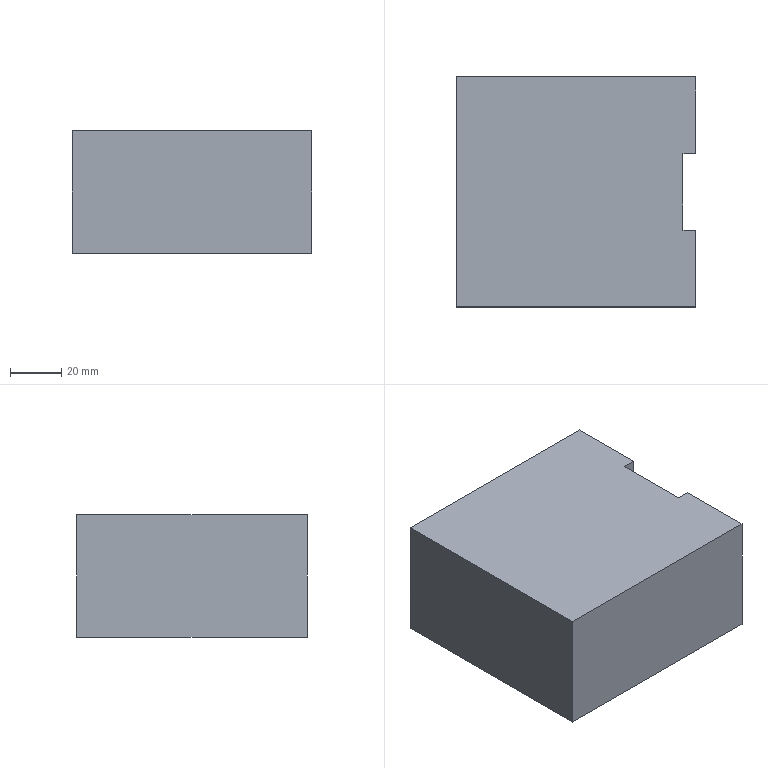Part | STEP file | plc | 1 solid | 10 faces | box 93.7 x 90 x 48.1 mm | volume 398412 mm3 | plane 10
STEP:
#1=CARTESIAN_POINT('',(0.,0.,0.));
#2=DIRECTION('',(0.,0.,1.));
#3=DIRECTION('',(1.,0.,0.));
#4=AXIS2_PLACEMENT_3D('',#1,#2,#3);
#5=CARTESIAN_POINT('',(46.85,-45.,0.));
#6=VERTEX_POINT('',#5);
#7=CARTESIAN_POINT('',(46.85,-15.,0.));
#8=VERTEX_POINT('',#7);
#9=CARTESIAN_POINT('',(46.85,45.,0.));
#10=DIRECTION('',(0.,1.,0.));
#11=VECTOR('',#10,1.);
#12=LINE('',#9,#11);
#13=CARTESIAN_POINT('',(46.85,45.,48.1));
#14=DIRECTION('',(-1.,0.,0.));
#15=DIRECTION('',(0.,-1.,0.));
#16=AXIS2_PLACEMENT_3D('',#13,#14,#15);
#17=PLANE('',#16);
#18=CARTESIAN_POINT('',(0.,-48.1));
#19=DIRECTION('',(-1.,0.));
#20=VECTOR('',#19,1.);
#21=LINE('',#18,#20);
#22=(GEOMETRIC_REPRESENTATION_CONTEXT(2)PARAMETRIC_REPRESENTATION_CONTEXT()REPRESENTATION_CONTEXT('',''));
#23=DEFINITIONAL_REPRESENTATION('',(#21),#22);
#24=PCURVE('',#17,#23);
#25=CARTESIAN_POINT('',(0.,0.,0.));
#26=DIRECTION('',(0.,0.,-1.));
#27=DIRECTION('',(-1.,0.,0.));
#28=AXIS2_PLACEMENT_3D('',#25,#26,#27);
#29=PLANE('',#28);
#30=CARTESIAN_POINT('',(-46.85,45.));
#31=DIRECTION('',(0.,1.));
#32=VECTOR('',#31,1.);
#33=LINE('',#30,#32);
#34=(GEOMETRIC_REPRESENTATION_CONTEXT(2)PARAMETRIC_REPRESENTATION_CONTEXT()REPRESENTATION_CONTEXT('',''));
#35=DEFINITIONAL_REPRESENTATION('',(#33),#34);
#36=PCURVE('',#29,#35);
#37=SURFACE_CURVE('',#12,(#24,#36),.PCURVE_S1.);
#38=EDGE_CURVE('',#6,#8,#37,.T.);
#39=ORIENTED_EDGE('',*,*,#38,.T.);
#40=CARTESIAN_POINT('',(46.85,-15.,48.1));
#41=VERTEX_POINT('',#40);
#42=CARTESIAN_POINT('',(46.85,-15.,0.));
#43=DIRECTION('',(0.,0.,1.));
#44=VECTOR('',#43,1.);
#45=LINE('',#42,#44);
#46=CARTESIAN_POINT('',(60.,-48.1));
#47=DIRECTION('',(0.,1.));
#48=VECTOR('',#47,1.);
#49=LINE('',#46,#48);
#50=(GEOMETRIC_REPRESENTATION_CONTEXT(2)PARAMETRIC_REPRESENTATION_CONTEXT()REPRESENTATION_CONTEXT('',''));
#51=DEFINITIONAL_REPRESENTATION('',(#49),#50);
#52=PCURVE('',#17,#51);
#53=CARTESIAN_POINT('',(46.85,-15.,0.));
#54=DIRECTION('',(0.,-1.,0.));
#55=DIRECTION('',(1.,0.,0.));
#56=AXIS2_PLACEMENT_3D('',#53,#54,#55);
#57=PLANE('',#56);
#58=CARTESIAN_POINT('',(0.,0.));
#59=DIRECTION('',(0.,1.));
#60=VECTOR('',#59,1.);
#61=LINE('',#58,#60);
#62=(GEOMETRIC_REPRESENTATION_CONTEXT(2)PARAMETRIC_REPRESENTATION_CONTEXT()REPRESENTATION_CONTEXT('',''));
#63=DEFINITIONAL_REPRESENTATION('',(#61),#62);
#64=PCURVE('',#57,#63);
#65=SURFACE_CURVE('',#45,(#52,#64),.PCURVE_S1.);
#66=EDGE_CURVE('',#8,#41,#65,.T.);
#67=ORIENTED_EDGE('',*,*,#66,.T.);
#68=CARTESIAN_POINT('',(46.85,-45.,48.1));
#69=VERTEX_POINT('',#68);
#70=CARTESIAN_POINT('',(46.85,45.,48.1));
#71=DIRECTION('',(0.,1.,0.));
#72=VECTOR('',#71,1.);
#73=LINE('',#70,#72);
#74=CARTESIAN_POINT('',(0.,0.));
#75=DIRECTION('',(-1.,0.));
#76=VECTOR('',#75,1.);
#77=LINE('',#74,#76);
#78=(GEOMETRIC_REPRESENTATION_CONTEXT(2)PARAMETRIC_REPRESENTATION_CONTEXT()REPRESENTATION_CONTEXT('',''));
#79=DEFINITIONAL_REPRESENTATION('',(#77),#78);
#80=PCURVE('',#17,#79);
#81=CARTESIAN_POINT('',(0.,0.,48.1));
#82=DIRECTION('',(0.,0.,-1.));
#83=DIRECTION('',(-1.,0.,0.));
#84=AXIS2_PLACEMENT_3D('',#81,#82,#83);
#85=PLANE('',#84);
#86=CARTESIAN_POINT('',(-46.85,45.));
#87=DIRECTION('',(0.,1.));
#88=VECTOR('',#87,1.);
#89=LINE('',#86,#88);
#90=(GEOMETRIC_REPRESENTATION_CONTEXT(2)PARAMETRIC_REPRESENTATION_CONTEXT()REPRESENTATION_CONTEXT('',''));
#91=DEFINITIONAL_REPRESENTATION('',(#89),#90);
#92=PCURVE('',#85,#91);
#93=SURFACE_CURVE('',#73,(#80,#92),.PCURVE_S1.);
#94=EDGE_CURVE('',#69,#41,#93,.T.);
#95=ORIENTED_EDGE('',*,*,#94,.F.);
#96=CARTESIAN_POINT('',(46.85,-45.,48.1));
#97=DIRECTION('',(0.,0.,-1.));
#98=VECTOR('',#97,1.);
#99=LINE('',#96,#98);
#100=CARTESIAN_POINT('',(90.,0.));
#101=DIRECTION('',(0.,-1.));
#102=VECTOR('',#101,1.);
#103=LINE('',#100,#102);
#104=(GEOMETRIC_REPRESENTATION_CONTEXT(2)PARAMETRIC_REPRESENTATION_CONTEXT()REPRESENTATION_CONTEXT('',''));
#105=DEFINITIONAL_REPRESENTATION('',(#103),#104);
#106=PCURVE('',#17,#105);
#107=CARTESIAN_POINT('',(46.85,-45.,48.1));
#108=DIRECTION('',(0.,1.,0.));
#109=DIRECTION('',(-1.,0.,0.));
#110=AXIS2_PLACEMENT_3D('',#107,#108,#109);
#111=PLANE('',#110);
#112=CARTESIAN_POINT('',(0.,0.));
#113=DIRECTION('',(0.,-1.));
#114=VECTOR('',#113,1.);
#115=LINE('',#112,#114);
#116=(GEOMETRIC_REPRESENTATION_CONTEXT(2)PARAMETRIC_REPRESENTATION_CONTEXT()REPRESENTATION_CONTEXT('',''));
#117=DEFINITIONAL_REPRESENTATION('',(#115),#116);
#118=PCURVE('',#111,#117);
#119=SURFACE_CURVE('',#99,(#106,#118),.PCURVE_S1.);
#120=EDGE_CURVE('',#69,#6,#119,.T.);
#121=ORIENTED_EDGE('',*,*,#120,.T.);
#122=EDGE_LOOP('',(#39,#67,#95,#121));
#123=FACE_BOUND('',#122,.T.);
#124=ADVANCED_FACE('',(#123),#17,.F.);
#125=CARTESIAN_POINT('',(-46.85,45.,0.));
#126=VERTEX_POINT('',#125);
#127=CARTESIAN_POINT('',(-46.85,-45.,0.));
#128=VERTEX_POINT('',#127);
#129=CARTESIAN_POINT('',(-46.85,45.,0.));
#130=DIRECTION('',(0.,-1.,0.));
#131=VECTOR('',#130,1.);
#132=LINE('',#129,#131);
#133=CARTESIAN_POINT('',(-46.85,45.,48.1));
#134=DIRECTION('',(1.,0.,0.));
#135=DIRECTION('',(0.,1.,0.));
#136=AXIS2_PLACEMENT_3D('',#133,#134,#135);
#137=PLANE('',#136);
#138=CARTESIAN_POINT('',(0.,-48.1));
#139=DIRECTION('',(-1.,0.));
#140=VECTOR('',#139,1.);
#141=LINE('',#138,#140);
#142=(GEOMETRIC_REPRESENTATION_CONTEXT(2)PARAMETRIC_REPRESENTATION_CONTEXT()REPRESENTATION_CONTEXT('',''));
#143=DEFINITIONAL_REPRESENTATION('',(#141),#142);
#144=PCURVE('',#137,#143);
#145=CARTESIAN_POINT('',(46.85,45.));
#146=DIRECTION('',(0.,-1.));
#147=VECTOR('',#146,1.);
#148=LINE('',#145,#147);
#149=(GEOMETRIC_REPRESENTATION_CONTEXT(2)PARAMETRIC_REPRESENTATION_CONTEXT()REPRESENTATION_CONTEXT('',''));
#150=DEFINITIONAL_REPRESENTATION('',(#148),#149);
#151=PCURVE('',#29,#150);
#152=SURFACE_CURVE('',#132,(#144,#151),.PCURVE_S1.);
#153=EDGE_CURVE('',#126,#128,#152,.T.);
#154=ORIENTED_EDGE('',*,*,#153,.T.);
#155=CARTESIAN_POINT('',(-46.85,-45.,48.1));
#156=VERTEX_POINT('',#155);
#157=CARTESIAN_POINT('',(-46.85,-45.,48.1));
#158=DIRECTION('',(0.,0.,-1.));
#159=VECTOR('',#158,1.);
#160=LINE('',#157,#159);
#161=CARTESIAN_POINT('',(-90.,0.));
#162=DIRECTION('',(0.,-1.));
#163=VECTOR('',#162,1.);
#164=LINE('',#161,#163);
#165=(GEOMETRIC_REPRESENTATION_CONTEXT(2)PARAMETRIC_REPRESENTATION_CONTEXT()REPRESENTATION_CONTEXT('',''));
#166=DEFINITIONAL_REPRESENTATION('',(#164),#165);
#167=PCURVE('',#137,#166);
#168=CARTESIAN_POINT('',(93.7,0.));
#169=DIRECTION('',(0.,-1.));
#170=VECTOR('',#169,1.);
#171=LINE('',#168,#170);
#172=(GEOMETRIC_REPRESENTATION_CONTEXT(2)PARAMETRIC_REPRESENTATION_CONTEXT()REPRESENTATION_CONTEXT('',''));
#173=DEFINITIONAL_REPRESENTATION('',(#171),#172);
#174=PCURVE('',#111,#173);
#175=SURFACE_CURVE('',#160,(#167,#174),.PCURVE_S1.);
#176=EDGE_CURVE('',#156,#128,#175,.T.);
#177=ORIENTED_EDGE('',*,*,#176,.F.);
#178=CARTESIAN_POINT('',(-46.85,45.,48.1));
#179=VERTEX_POINT('',#178);
#180=CARTESIAN_POINT('',(-46.85,45.,48.1));
#181=DIRECTION('',(0.,-1.,0.));
#182=VECTOR('',#181,1.);
#183=LINE('',#180,#182);
#184=CARTESIAN_POINT('',(0.,0.));
#185=DIRECTION('',(-1.,0.));
#186=VECTOR('',#185,1.);
#187=LINE('',#184,#186);
#188=(GEOMETRIC_REPRESENTATION_CONTEXT(2)PARAMETRIC_REPRESENTATION_CONTEXT()REPRESENTATION_CONTEXT('',''));
#189=DEFINITIONAL_REPRESENTATION('',(#187),#188);
#190=PCURVE('',#137,#189);
#191=CARTESIAN_POINT('',(46.85,45.));
#192=DIRECTION('',(0.,-1.));
#193=VECTOR('',#192,1.);
#194=LINE('',#191,#193);
#195=(GEOMETRIC_REPRESENTATION_CONTEXT(2)PARAMETRIC_REPRESENTATION_CONTEXT()REPRESENTATION_CONTEXT('',''));
#196=DEFINITIONAL_REPRESENTATION('',(#194),#195);
#197=PCURVE('',#85,#196);
#198=SURFACE_CURVE('',#183,(#190,#197),.PCURVE_S1.);
#199=EDGE_CURVE('',#179,#156,#198,.T.);
#200=ORIENTED_EDGE('',*,*,#199,.F.);
#201=CARTESIAN_POINT('',(-46.85,45.,48.1));
#202=DIRECTION('',(0.,0.,-1.));
#203=VECTOR('',#202,1.);
#204=LINE('',#201,#203);
#205=CARTESIAN_POINT('',(0.,0.));
#206=DIRECTION('',(0.,-1.));
#207=VECTOR('',#206,1.);
#208=LINE('',#205,#207);
#209=(GEOMETRIC_REPRESENTATION_CONTEXT(2)PARAMETRIC_REPRESENTATION_CONTEXT()REPRESENTATION_CONTEXT('',''));
#210=DEFINITIONAL_REPRESENTATION('',(#208),#209);
#211=PCURVE('',#137,#210);
#212=CARTESIAN_POINT('',(46.85,45.,48.1));
#213=DIRECTION('',(0.,-1.,0.));
#214=DIRECTION('',(1.,0.,0.));
#215=AXIS2_PLACEMENT_3D('',#212,#213,#214);
#216=PLANE('',#215);
#217=CARTESIAN_POINT('',(-93.7,0.));
#218=DIRECTION('',(0.,-1.));
#219=VECTOR('',#218,1.);
#220=LINE('',#217,#219);
#221=(GEOMETRIC_REPRESENTATION_CONTEXT(2)PARAMETRIC_REPRESENTATION_CONTEXT()REPRESENTATION_CONTEXT('',''));
#222=DEFINITIONAL_REPRESENTATION('',(#220),#221);
#223=PCURVE('',#216,#222);
#224=SURFACE_CURVE('',#204,(#211,#223),.PCURVE_S1.);
#225=EDGE_CURVE('',#179,#126,#224,.T.);
#226=ORIENTED_EDGE('',*,*,#225,.T.);
#227=EDGE_LOOP('',(#154,#177,#200,#226));
#228=FACE_BOUND('',#227,.T.);
#229=ADVANCED_FACE('',(#228),#137,.F.);
#230=CARTESIAN_POINT('',(46.85,-45.,0.));
#231=DIRECTION('',(1.,0.,0.));
#232=VECTOR('',#231,1.);
#233=LINE('',#230,#232);
#234=CARTESIAN_POINT('',(0.,-48.1));
#235=DIRECTION('',(-1.,0.));
#236=VECTOR('',#235,1.);
#237=LINE('',#234,#236);
#238=(GEOMETRIC_REPRESENTATION_CONTEXT(2)PARAMETRIC_REPRESENTATION_CONTEXT()REPRESENTATION_CONTEXT('',''));
#239=DEFINITIONAL_REPRESENTATION('',(#237),#238);
#240=PCURVE('',#111,#239);
#241=CARTESIAN_POINT('',(-46.85,-45.));
#242=DIRECTION('',(-1.,0.));
#243=VECTOR('',#242,1.);
#244=LINE('',#241,#243);
#245=(GEOMETRIC_REPRESENTATION_CONTEXT(2)PARAMETRIC_REPRESENTATION_CONTEXT()REPRESENTATION_CONTEXT('',''));
#246=DEFINITIONAL_REPRESENTATION('',(#244),#245);
#247=PCURVE('',#29,#246);
#248=SURFACE_CURVE('',#233,(#240,#247),.PCURVE_S1.);
#249=EDGE_CURVE('',#128,#6,#248,.T.);
#250=ORIENTED_EDGE('',*,*,#249,.T.);
#251=ORIENTED_EDGE('',*,*,#120,.F.);
#252=CARTESIAN_POINT('',(46.85,-45.,48.1));
#253=DIRECTION('',(1.,0.,0.));
#254=VECTOR('',#253,1.);
#255=LINE('',#252,#254);
#256=CARTESIAN_POINT('',(0.,0.));
#257=DIRECTION('',(-1.,0.));
#258=VECTOR('',#257,1.);
#259=LINE('',#256,#258);
#260=(GEOMETRIC_REPRESENTATION_CONTEXT(2)PARAMETRIC_REPRESENTATION_CONTEXT()REPRESENTATION_CONTEXT('',''));
#261=DEFINITIONAL_REPRESENTATION('',(#259),#260);
#262=PCURVE('',#111,#261);
#263=CARTESIAN_POINT('',(-46.85,-45.));
#264=DIRECTION('',(-1.,0.));
#265=VECTOR('',#264,1.);
#266=LINE('',#263,#265);
#267=(GEOMETRIC_REPRESENTATION_CONTEXT(2)PARAMETRIC_REPRESENTATION_CONTEXT()REPRESENTATION_CONTEXT('',''));
#268=DEFINITIONAL_REPRESENTATION('',(#266),#267);
#269=PCURVE('',#85,#268);
#270=SURFACE_CURVE('',#255,(#262,#269),.PCURVE_S1.);
#271=EDGE_CURVE('',#156,#69,#270,.T.);
#272=ORIENTED_EDGE('',*,*,#271,.F.);
#273=ORIENTED_EDGE('',*,*,#176,.T.);
#274=EDGE_LOOP('',(#250,#251,#272,#273));
#275=FACE_BOUND('',#274,.T.);
#276=ADVANCED_FACE('',(#275),#111,.F.);
#277=CARTESIAN_POINT('',(46.85,15.,48.1));
#278=VERTEX_POINT('',#277);
#279=CARTESIAN_POINT('',(46.85,45.,48.1));
#280=VERTEX_POINT('',#279);
#281=CARTESIAN_POINT('',(46.85,45.,48.1));
#282=DIRECTION('',(0.,1.,0.));
#283=VECTOR('',#282,1.);
#284=LINE('',#281,#283);
#285=CARTESIAN_POINT('',(46.85,45.,48.1));
#286=DIRECTION('',(-1.,0.,0.));
#287=DIRECTION('',(0.,-1.,0.));
#288=AXIS2_PLACEMENT_3D('',#285,#286,#287);
#289=PLANE('',#288);
#290=CARTESIAN_POINT('',(0.,0.));
#291=DIRECTION('',(-1.,0.));
#292=VECTOR('',#291,1.);
#293=LINE('',#290,#292);
#294=(GEOMETRIC_REPRESENTATION_CONTEXT(2)PARAMETRIC_REPRESENTATION_CONTEXT()REPRESENTATION_CONTEXT('',''));
#295=DEFINITIONAL_REPRESENTATION('',(#293),#294);
#296=PCURVE('',#289,#295);
#297=CARTESIAN_POINT('',(-46.85,45.));
#298=DIRECTION('',(0.,1.));
#299=VECTOR('',#298,1.);
#300=LINE('',#297,#299);
#301=(GEOMETRIC_REPRESENTATION_CONTEXT(2)PARAMETRIC_REPRESENTATION_CONTEXT()REPRESENTATION_CONTEXT('',''));
#302=DEFINITIONAL_REPRESENTATION('',(#300),#301);
#303=PCURVE('',#85,#302);
#304=SURFACE_CURVE('',#284,(#296,#303),.PCURVE_S1.);
#305=EDGE_CURVE('',#278,#280,#304,.T.);
#306=ORIENTED_EDGE('',*,*,#305,.F.);
#307=CARTESIAN_POINT('',(46.85,15.,0.));
#308=VERTEX_POINT('',#307);
#309=CARTESIAN_POINT('',(46.85,15.,0.));
#310=DIRECTION('',(0.,0.,1.));
#311=VECTOR('',#310,1.);
#312=LINE('',#309,#311);
#313=CARTESIAN_POINT('',(30.,-48.1));
#314=DIRECTION('',(0.,1.));
#315=VECTOR('',#314,1.);
#316=LINE('',#313,#315);
#317=(GEOMETRIC_REPRESENTATION_CONTEXT(2)PARAMETRIC_REPRESENTATION_CONTEXT()REPRESENTATION_CONTEXT('',''));
#318=DEFINITIONAL_REPRESENTATION('',(#316),#317);
#319=PCURVE('',#289,#318);
#320=CARTESIAN_POINT('',(46.85,15.,0.));
#321=DIRECTION('',(0.,1.,0.));
#322=DIRECTION('',(-1.,0.,0.));
#323=AXIS2_PLACEMENT_3D('',#320,#321,#322);
#324=PLANE('',#323);
#325=CARTESIAN_POINT('',(0.,0.));
#326=DIRECTION('',(0.,1.));
#327=VECTOR('',#326,1.);
#328=LINE('',#325,#327);
#329=(GEOMETRIC_REPRESENTATION_CONTEXT(2)PARAMETRIC_REPRESENTATION_CONTEXT()REPRESENTATION_CONTEXT('',''));
#330=DEFINITIONAL_REPRESENTATION('',(#328),#329);
#331=PCURVE('',#324,#330);
#332=SURFACE_CURVE('',#312,(#319,#331),.PCURVE_S1.);
#333=EDGE_CURVE('',#308,#278,#332,.T.);
#334=ORIENTED_EDGE('',*,*,#333,.F.);
#335=CARTESIAN_POINT('',(46.85,45.,0.));
#336=VERTEX_POINT('',#335);
#337=CARTESIAN_POINT('',(46.85,45.,0.));
#338=DIRECTION('',(0.,1.,0.));
#339=VECTOR('',#338,1.);
#340=LINE('',#337,#339);
#341=CARTESIAN_POINT('',(0.,-48.1));
#342=DIRECTION('',(-1.,0.));
#343=VECTOR('',#342,1.);
#344=LINE('',#341,#343);
#345=(GEOMETRIC_REPRESENTATION_CONTEXT(2)PARAMETRIC_REPRESENTATION_CONTEXT()REPRESENTATION_CONTEXT('',''));
#346=DEFINITIONAL_REPRESENTATION('',(#344),#345);
#347=PCURVE('',#289,#346);
#348=CARTESIAN_POINT('',(-46.85,45.));
#349=DIRECTION('',(0.,1.));
#350=VECTOR('',#349,1.);
#351=LINE('',#348,#350);
#352=(GEOMETRIC_REPRESENTATION_CONTEXT(2)PARAMETRIC_REPRESENTATION_CONTEXT()REPRESENTATION_CONTEXT('',''));
#353=DEFINITIONAL_REPRESENTATION('',(#351),#352);
#354=PCURVE('',#29,#353);
#355=SURFACE_CURVE('',#340,(#347,#354),.PCURVE_S1.);
#356=EDGE_CURVE('',#308,#336,#355,.T.);
#357=ORIENTED_EDGE('',*,*,#356,.T.);
#358=CARTESIAN_POINT('',(46.85,45.,48.1));
#359=DIRECTION('',(0.,0.,-1.));
#360=VECTOR('',#359,1.);
#361=LINE('',#358,#360);
#362=CARTESIAN_POINT('',(0.,0.));
#363=DIRECTION('',(0.,-1.));
#364=VECTOR('',#363,1.);
#365=LINE('',#362,#364);
#366=(GEOMETRIC_REPRESENTATION_CONTEXT(2)PARAMETRIC_REPRESENTATION_CONTEXT()REPRESENTATION_CONTEXT('',''));
#367=DEFINITIONAL_REPRESENTATION('',(#365),#366);
#368=PCURVE('',#289,#367);
#369=CARTESIAN_POINT('',(0.,0.));
#370=DIRECTION('',(0.,-1.));
#371=VECTOR('',#370,1.);
#372=LINE('',#369,#371);
#373=(GEOMETRIC_REPRESENTATION_CONTEXT(2)PARAMETRIC_REPRESENTATION_CONTEXT()REPRESENTATION_CONTEXT('',''));
#374=DEFINITIONAL_REPRESENTATION('',(#372),#373);
#375=PCURVE('',#216,#374);
#376=SURFACE_CURVE('',#361,(#368,#375),.PCURVE_S1.);
#377=EDGE_CURVE('',#280,#336,#376,.T.);
#378=ORIENTED_EDGE('',*,*,#377,.F.);
#379=EDGE_LOOP('',(#306,#334,#357,#378));
#380=FACE_BOUND('',#379,.T.);
#381=ADVANCED_FACE('',(#380),#289,.F.);
#382=CARTESIAN_POINT('',(46.85,45.,0.));
#383=DIRECTION('',(-1.,0.,0.));
#384=VECTOR('',#383,1.);
#385=LINE('',#382,#384);
#386=CARTESIAN_POINT('',(0.,-48.1));
#387=DIRECTION('',(-1.,0.));
#388=VECTOR('',#387,1.);
#389=LINE('',#386,#388);
#390=(GEOMETRIC_REPRESENTATION_CONTEXT(2)PARAMETRIC_REPRESENTATION_CONTEXT()REPRESENTATION_CONTEXT('',''));
#391=DEFINITIONAL_REPRESENTATION('',(#389),#390);
#392=PCURVE('',#216,#391);
#393=CARTESIAN_POINT('',(-46.85,45.));
#394=DIRECTION('',(1.,0.));
#395=VECTOR('',#394,1.);
#396=LINE('',#393,#395);
#397=(GEOMETRIC_REPRESENTATION_CONTEXT(2)PARAMETRIC_REPRESENTATION_CONTEXT()REPRESENTATION_CONTEXT('',''));
#398=DEFINITIONAL_REPRESENTATION('',(#396),#397);
#399=PCURVE('',#29,#398);
#400=SURFACE_CURVE('',#385,(#392,#399),.PCURVE_S1.);
#401=EDGE_CURVE('',#336,#126,#400,.T.);
#402=ORIENTED_EDGE('',*,*,#401,.T.);
#403=ORIENTED_EDGE('',*,*,#225,.F.);
#404=CARTESIAN_POINT('',(46.85,45.,48.1));
#405=DIRECTION('',(-1.,0.,0.));
#406=VECTOR('',#405,1.);
#407=LINE('',#404,#406);
#408=CARTESIAN_POINT('',(0.,0.));
#409=DIRECTION('',(-1.,0.));
#410=VECTOR('',#409,1.);
#411=LINE('',#408,#410);
#412=(GEOMETRIC_REPRESENTATION_CONTEXT(2)PARAMETRIC_REPRESENTATION_CONTEXT()REPRESENTATION_CONTEXT('',''));
#413=DEFINITIONAL_REPRESENTATION('',(#411),#412);
#414=PCURVE('',#216,#413);
#415=CARTESIAN_POINT('',(-46.85,45.));
#416=DIRECTION('',(1.,0.));
#417=VECTOR('',#416,1.);
#418=LINE('',#415,#417);
#419=(GEOMETRIC_REPRESENTATION_CONTEXT(2)PARAMETRIC_REPRESENTATION_CONTEXT()REPRESENTATION_CONTEXT('',''));
#420=DEFINITIONAL_REPRESENTATION('',(#418),#419);
#421=PCURVE('',#85,#420);
#422=SURFACE_CURVE('',#407,(#414,#421),.PCURVE_S1.);
#423=EDGE_CURVE('',#280,#179,#422,.T.);
#424=ORIENTED_EDGE('',*,*,#423,.F.);
#425=ORIENTED_EDGE('',*,*,#377,.T.);
#426=EDGE_LOOP('',(#402,#403,#424,#425));
#427=FACE_BOUND('',#426,.T.);
#428=ADVANCED_FACE('',(#427),#216,.F.);
#429=ORIENTED_EDGE('',*,*,#94,.T.);
#430=CARTESIAN_POINT('',(41.85,-15.,48.1));
#431=VERTEX_POINT('',#430);
#432=CARTESIAN_POINT('',(46.85,-15.,48.1));
#433=DIRECTION('',(1.,0.,0.));
#434=VECTOR('',#433,1.);
#435=LINE('',#432,#434);
#436=CARTESIAN_POINT('',(-46.85,-15.));
#437=DIRECTION('',(-1.,0.));
#438=VECTOR('',#437,1.);
#439=LINE('',#436,#438);
#440=(GEOMETRIC_REPRESENTATION_CONTEXT(2)PARAMETRIC_REPRESENTATION_CONTEXT()REPRESENTATION_CONTEXT('',''));
#441=DEFINITIONAL_REPRESENTATION('',(#439),#440);
#442=PCURVE('',#85,#441);
#443=CARTESIAN_POINT('',(0.,48.1));
#444=DIRECTION('',(1.,0.));
#445=VECTOR('',#444,1.);
#446=LINE('',#443,#445);
#447=(GEOMETRIC_REPRESENTATION_CONTEXT(2)PARAMETRIC_REPRESENTATION_CONTEXT()REPRESENTATION_CONTEXT('',''));
#448=DEFINITIONAL_REPRESENTATION('',(#446),#447);
#449=PCURVE('',#57,#448);
#450=SURFACE_CURVE('',#435,(#442,#449),.PCURVE_S1.);
#451=EDGE_CURVE('',#431,#41,#450,.T.);
#452=ORIENTED_EDGE('',*,*,#451,.F.);
#453=CARTESIAN_POINT('',(41.85,15.,48.1));
#454=VERTEX_POINT('',#453);
#455=CARTESIAN_POINT('',(41.85,-15.,48.1));
#456=DIRECTION('',(0.,-1.,0.));
#457=VECTOR('',#456,1.);
#458=LINE('',#455,#457);
#459=CARTESIAN_POINT('',(-41.85,-15.));
#460=DIRECTION('',(0.,-1.));
#461=VECTOR('',#460,1.);
#462=LINE('',#459,#461);
#463=(GEOMETRIC_REPRESENTATION_CONTEXT(2)PARAMETRIC_REPRESENTATION_CONTEXT()REPRESENTATION_CONTEXT('',''));
#464=DEFINITIONAL_REPRESENTATION('',(#462),#463);
#465=PCURVE('',#85,#464);
#466=CARTESIAN_POINT('',(41.85,-15.,0.));
#467=DIRECTION('',(-1.,0.,0.));
#468=DIRECTION('',(0.,0.,1.));
#469=AXIS2_PLACEMENT_3D('',#466,#467,#468);
#470=PLANE('',#469);
#471=CARTESIAN_POINT('',(48.1,0.));
#472=DIRECTION('',(0.,-1.));
#473=VECTOR('',#472,1.);
#474=LINE('',#471,#473);
#475=(GEOMETRIC_REPRESENTATION_CONTEXT(2)PARAMETRIC_REPRESENTATION_CONTEXT()REPRESENTATION_CONTEXT('',''));
#476=DEFINITIONAL_REPRESENTATION('',(#474),#475);
#477=PCURVE('',#470,#476);
#478=SURFACE_CURVE('',#458,(#465,#477),.PCURVE_S1.);
#479=EDGE_CURVE('',#454,#431,#478,.T.);
#480=ORIENTED_EDGE('',*,*,#479,.F.);
#481=CARTESIAN_POINT('',(46.85,15.,48.1));
#482=DIRECTION('',(-1.,0.,0.));
#483=VECTOR('',#482,1.);
#484=LINE('',#481,#483);
#485=CARTESIAN_POINT('',(-46.85,15.));
#486=DIRECTION('',(1.,0.));
#487=VECTOR('',#486,1.);
#488=LINE('',#485,#487);
#489=(GEOMETRIC_REPRESENTATION_CONTEXT(2)PARAMETRIC_REPRESENTATION_CONTEXT()REPRESENTATION_CONTEXT('',''));
#490=DEFINITIONAL_REPRESENTATION('',(#488),#489);
#491=PCURVE('',#85,#490);
#492=CARTESIAN_POINT('',(0.,48.1));
#493=DIRECTION('',(1.,0.));
#494=VECTOR('',#493,1.);
#495=LINE('',#492,#494);
#496=(GEOMETRIC_REPRESENTATION_CONTEXT(2)PARAMETRIC_REPRESENTATION_CONTEXT()REPRESENTATION_CONTEXT('',''));
#497=DEFINITIONAL_REPRESENTATION('',(#495),#496);
#498=PCURVE('',#324,#497);
#499=SURFACE_CURVE('',#484,(#491,#498),.PCURVE_S1.);
#500=EDGE_CURVE('',#278,#454,#499,.T.);
#501=ORIENTED_EDGE('',*,*,#500,.F.);
#502=ORIENTED_EDGE('',*,*,#305,.T.);
#503=ORIENTED_EDGE('',*,*,#423,.T.);
#504=ORIENTED_EDGE('',*,*,#199,.T.);
#505=ORIENTED_EDGE('',*,*,#271,.T.);
#506=EDGE_LOOP('',(#429,#452,#480,#501,#502,#503,#504,#505));
#507=FACE_BOUND('',#506,.T.);
#508=ADVANCED_FACE('',(#507),#85,.F.);
#509=CARTESIAN_POINT('',(41.85,-15.,0.));
#510=VERTEX_POINT('',#509);
#511=CARTESIAN_POINT('',(46.85,-15.,0.));
#512=DIRECTION('',(1.,0.,0.));
#513=VECTOR('',#512,1.);
#514=LINE('',#511,#513);
#515=CARTESIAN_POINT('',(-46.85,-15.));
#516=DIRECTION('',(-1.,0.));
#517=VECTOR('',#516,1.);
#518=LINE('',#515,#517);
#519=(GEOMETRIC_REPRESENTATION_CONTEXT(2)PARAMETRIC_REPRESENTATION_CONTEXT()REPRESENTATION_CONTEXT('',''));
#520=DEFINITIONAL_REPRESENTATION('',(#518),#519);
#521=PCURVE('',#29,#520);
#522=CARTESIAN_POINT('',(0.,0.));
#523=DIRECTION('',(1.,0.));
#524=VECTOR('',#523,1.);
#525=LINE('',#522,#524);
#526=(GEOMETRIC_REPRESENTATION_CONTEXT(2)PARAMETRIC_REPRESENTATION_CONTEXT()REPRESENTATION_CONTEXT('',''));
#527=DEFINITIONAL_REPRESENTATION('',(#525),#526);
#528=PCURVE('',#57,#527);
#529=SURFACE_CURVE('',#514,(#521,#528),.PCURVE_S1.);
#530=EDGE_CURVE('',#510,#8,#529,.T.);
#531=ORIENTED_EDGE('',*,*,#530,.T.);
#532=ORIENTED_EDGE('',*,*,#38,.F.);
#533=ORIENTED_EDGE('',*,*,#249,.F.);
#534=ORIENTED_EDGE('',*,*,#153,.F.);
#535=ORIENTED_EDGE('',*,*,#401,.F.);
#536=ORIENTED_EDGE('',*,*,#356,.F.);
#537=CARTESIAN_POINT('',(41.85,15.,0.));
#538=VERTEX_POINT('',#537);
#539=CARTESIAN_POINT('',(46.85,15.,0.));
#540=DIRECTION('',(-1.,0.,0.));
#541=VECTOR('',#540,1.);
#542=LINE('',#539,#541);
#543=CARTESIAN_POINT('',(-46.85,15.));
#544=DIRECTION('',(1.,0.));
#545=VECTOR('',#544,1.);
#546=LINE('',#543,#545);
#547=(GEOMETRIC_REPRESENTATION_CONTEXT(2)PARAMETRIC_REPRESENTATION_CONTEXT()REPRESENTATION_CONTEXT('',''));
#548=DEFINITIONAL_REPRESENTATION('',(#546),#547);
#549=PCURVE('',#29,#548);
#550=CARTESIAN_POINT('',(0.,0.));
#551=DIRECTION('',(1.,0.));
#552=VECTOR('',#551,1.);
#553=LINE('',#550,#552);
#554=(GEOMETRIC_REPRESENTATION_CONTEXT(2)PARAMETRIC_REPRESENTATION_CONTEXT()REPRESENTATION_CONTEXT('',''));
#555=DEFINITIONAL_REPRESENTATION('',(#553),#554);
#556=PCURVE('',#324,#555);
#557=SURFACE_CURVE('',#542,(#549,#556),.PCURVE_S1.);
#558=EDGE_CURVE('',#308,#538,#557,.T.);
#559=ORIENTED_EDGE('',*,*,#558,.T.);
#560=CARTESIAN_POINT('',(41.85,-15.,0.));
#561=DIRECTION('',(0.,-1.,0.));
#562=VECTOR('',#561,1.);
#563=LINE('',#560,#562);
#564=CARTESIAN_POINT('',(-41.85,-15.));
#565=DIRECTION('',(0.,-1.));
#566=VECTOR('',#565,1.);
#567=LINE('',#564,#566);
#568=(GEOMETRIC_REPRESENTATION_CONTEXT(2)PARAMETRIC_REPRESENTATION_CONTEXT()REPRESENTATION_CONTEXT('',''));
#569=DEFINITIONAL_REPRESENTATION('',(#567),#568);
#570=PCURVE('',#29,#569);
#571=CARTESIAN_POINT('',(0.,0.));
#572=DIRECTION('',(0.,-1.));
#573=VECTOR('',#572,1.);
#574=LINE('',#571,#573);
#575=(GEOMETRIC_REPRESENTATION_CONTEXT(2)PARAMETRIC_REPRESENTATION_CONTEXT()REPRESENTATION_CONTEXT('',''));
#576=DEFINITIONAL_REPRESENTATION('',(#574),#575);
#577=PCURVE('',#470,#576);
#578=SURFACE_CURVE('',#563,(#570,#577),.PCURVE_S1.);
#579=EDGE_CURVE('',#538,#510,#578,.T.);
#580=ORIENTED_EDGE('',*,*,#579,.T.);
#581=EDGE_LOOP('',(#531,#532,#533,#534,#535,#536,#559,#580));
#582=FACE_BOUND('',#581,.T.);
#583=ADVANCED_FACE('',(#582),#29,.T.);
#584=ORIENTED_EDGE('',*,*,#451,.T.);
#585=ORIENTED_EDGE('',*,*,#66,.F.);
#586=ORIENTED_EDGE('',*,*,#530,.F.);
#587=CARTESIAN_POINT('',(41.85,-15.,0.));
#588=DIRECTION('',(0.,0.,1.));
#589=VECTOR('',#588,1.);
#590=LINE('',#587,#589);
#591=CARTESIAN_POINT('',(-5.,0.));
#592=DIRECTION('',(0.,1.));
#593=VECTOR('',#592,1.);
#594=LINE('',#591,#593);
#595=(GEOMETRIC_REPRESENTATION_CONTEXT(2)PARAMETRIC_REPRESENTATION_CONTEXT()REPRESENTATION_CONTEXT('',''));
#596=DEFINITIONAL_REPRESENTATION('',(#594),#595);
#597=PCURVE('',#57,#596);
#598=CARTESIAN_POINT('',(0.,0.));
#599=DIRECTION('',(1.,0.));
#600=VECTOR('',#599,1.);
#601=LINE('',#598,#600);
#602=(GEOMETRIC_REPRESENTATION_CONTEXT(2)PARAMETRIC_REPRESENTATION_CONTEXT()REPRESENTATION_CONTEXT('',''));
#603=DEFINITIONAL_REPRESENTATION('',(#601),#602);
#604=PCURVE('',#470,#603);
#605=SURFACE_CURVE('',#590,(#597,#604),.PCURVE_S1.);
#606=EDGE_CURVE('',#510,#431,#605,.T.);
#607=ORIENTED_EDGE('',*,*,#606,.T.);
#608=EDGE_LOOP('',(#584,#585,#586,#607));
#609=FACE_BOUND('',#608,.T.);
#610=ADVANCED_FACE('',(#609),#57,.F.);
#611=ORIENTED_EDGE('',*,*,#479,.T.);
#612=ORIENTED_EDGE('',*,*,#606,.F.);
#613=ORIENTED_EDGE('',*,*,#579,.F.);
#614=CARTESIAN_POINT('',(41.85,15.,0.));
#615=DIRECTION('',(0.,0.,1.));
#616=VECTOR('',#615,1.);
#617=LINE('',#614,#616);
#618=CARTESIAN_POINT('',(0.,30.));
#619=DIRECTION('',(1.,0.));
#620=VECTOR('',#619,1.);
#621=LINE('',#618,#620);
#622=(GEOMETRIC_REPRESENTATION_CONTEXT(2)PARAMETRIC_REPRESENTATION_CONTEXT()REPRESENTATION_CONTEXT('',''));
#623=DEFINITIONAL_REPRESENTATION('',(#621),#622);
#624=PCURVE('',#470,#623);
#625=CARTESIAN_POINT('',(5.,0.));
#626=DIRECTION('',(0.,1.));
#627=VECTOR('',#626,1.);
#628=LINE('',#625,#627);
#629=(GEOMETRIC_REPRESENTATION_CONTEXT(2)PARAMETRIC_REPRESENTATION_CONTEXT()REPRESENTATION_CONTEXT('',''));
#630=DEFINITIONAL_REPRESENTATION('',(#628),#629);
#631=PCURVE('',#324,#630);
#632=SURFACE_CURVE('',#617,(#624,#631),.PCURVE_S1.);
#633=EDGE_CURVE('',#538,#454,#632,.T.);
#634=ORIENTED_EDGE('',*,*,#633,.T.);
#635=EDGE_LOOP('',(#611,#612,#613,#634));
#636=FACE_BOUND('',#635,.T.);
#637=ADVANCED_FACE('',(#636),#470,.F.);
#638=ORIENTED_EDGE('',*,*,#500,.T.);
#639=ORIENTED_EDGE('',*,*,#633,.F.);
#640=ORIENTED_EDGE('',*,*,#558,.F.);
#641=ORIENTED_EDGE('',*,*,#333,.T.);
#642=EDGE_LOOP('',(#638,#639,#640,#641));
#643=FACE_BOUND('',#642,.T.);
#644=ADVANCED_FACE('',(#643),#324,.F.);
#645=CLOSED_SHELL('',(#124,#229,#276,#381,#428,#508,#583,#610,#637,#644));
#646=MANIFOLD_SOLID_BREP('',#645);
#647=(LENGTH_UNIT()NAMED_UNIT(*)SI_UNIT(.MILLI.,.METRE.));
#648=UNCERTAINTY_MEASURE_WITH_UNIT(LENGTH_MEASURE(0.0000001),#647,'','');
#649=(NAMED_UNIT(*)PLANE_ANGLE_UNIT()SI_UNIT($,.RADIAN.));
#650=(NAMED_UNIT(*)SI_UNIT($,.STERADIAN.)SOLID_ANGLE_UNIT());
#651=(GEOMETRIC_REPRESENTATION_CONTEXT(3)GLOBAL_UNCERTAINTY_ASSIGNED_CONTEXT((#648))GLOBAL_UNIT_ASSIGNED_CONTEXT((#647,#649,#650))REPRESENTATION_CONTEXT('',''));
#652=ADVANCED_BREP_SHAPE_REPRESENTATION('',(#4,#646),#651);